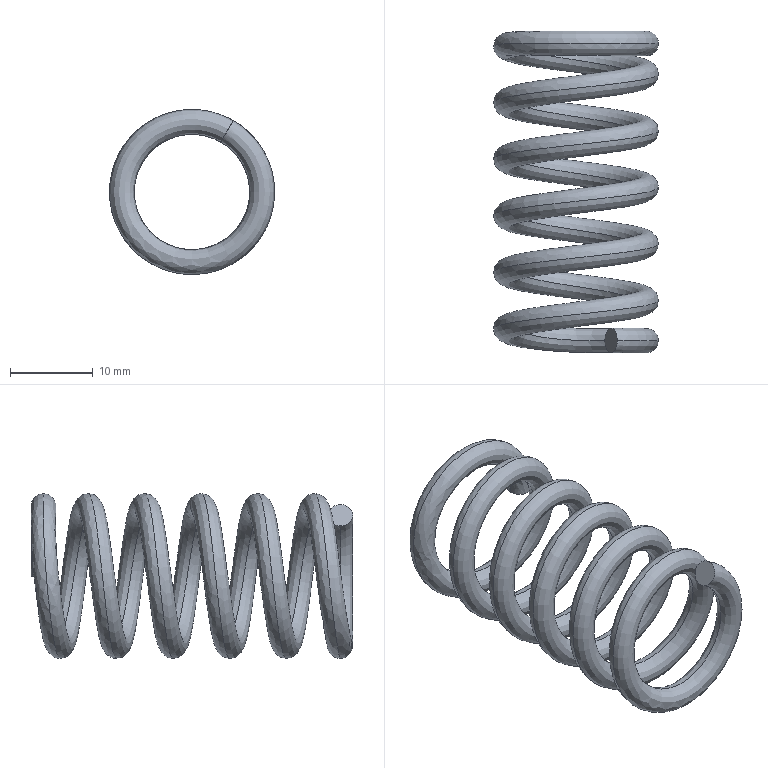Part | STEP file | LO XO D20d3X36 | 1 solid | 4 faces | box 20.006 x 39.001 x 20.006 mm | volume 2345 mm3 | spline 2 | plane 2